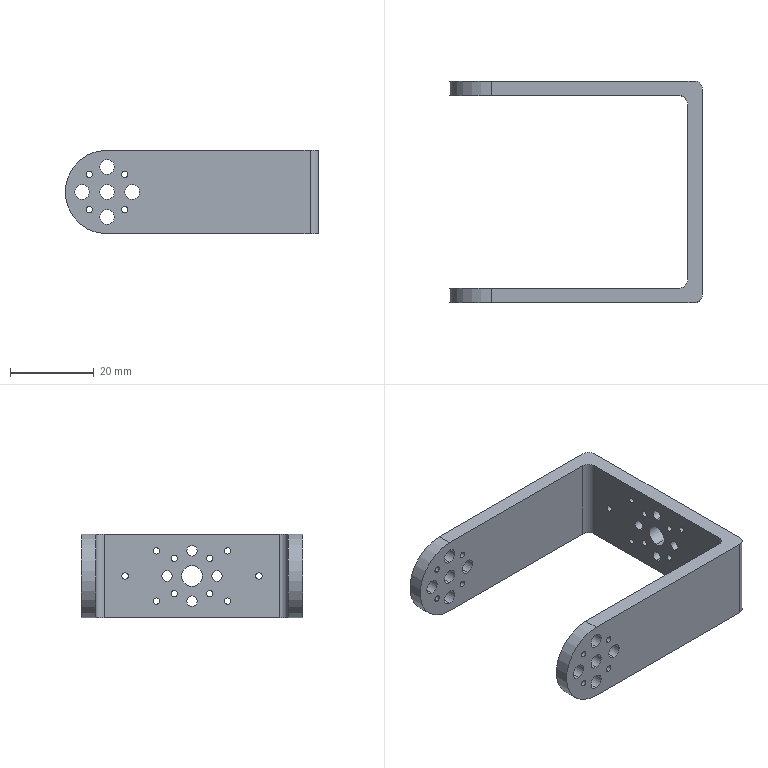Part | SolidWorks | features Cut 5, Fillet 2, Extrusion 1 | 1 solid | 80 faces | box 60.5 x 53 x 20 mm | volume 10804 mm3 | cylinder 72 | plane 8 | commonest cylinder face diameters 1.5 x36 3.5 x20 2.5 x8 4 x4 5 x2 20 x2